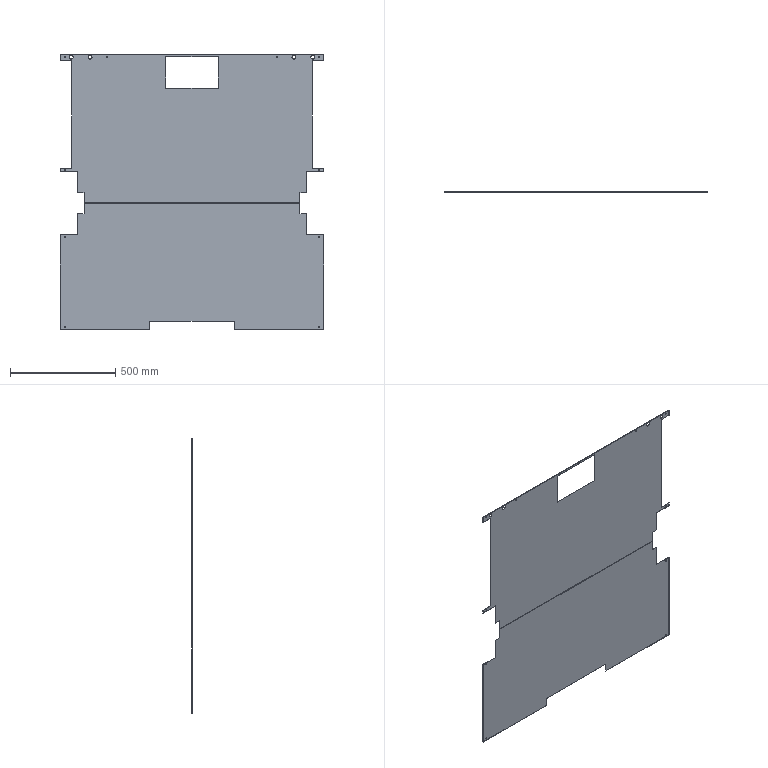Part | SolidWorks | features ICE 10, FlatPattern 2, SMBaseFlange 1, SheetMetal 1 | 2 solids | 72 faces | box 1250 x 1 x 1306 mm | volume 1467099 mm3 | plane 44 | cylinder 28 | commonest cylinder face diameters 5 x20 18 x8